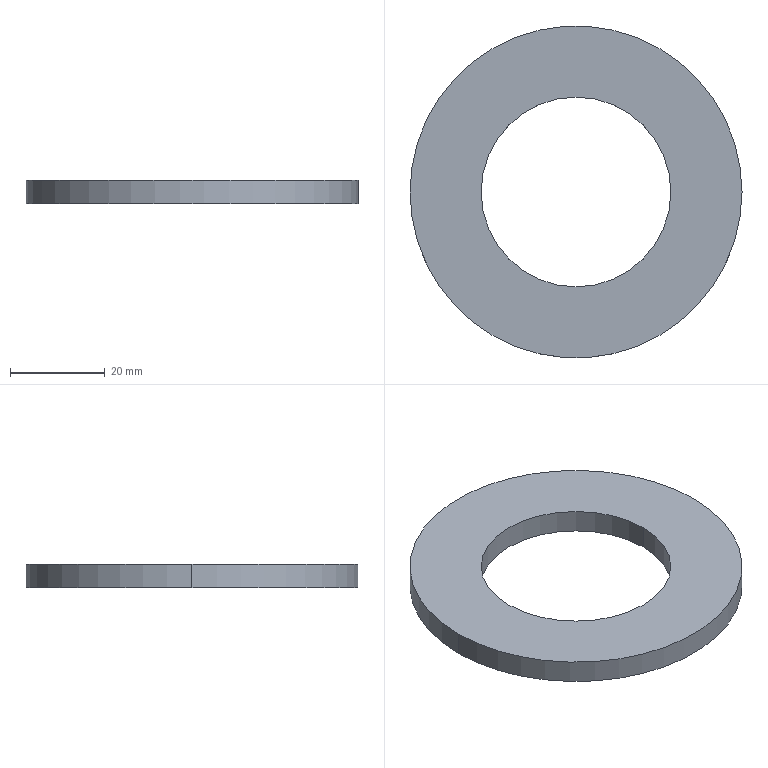Part | STEP file | 40 spacer XG | 1 solid | 6 faces | box 70 x 70 x 5 mm | volume 12959 mm3 | cylinder 4 | plane 2 | commonest cylinder face diameters 40 x2 70 x2
STEP:
#1=CARTESIAN_POINT('',(0.,0.,0.));
#2=DIRECTION('',(0.,0.,1.));
#3=DIRECTION('',(1.,0.,0.));
#4=AXIS2_PLACEMENT_3D('',#1,#2,#3);
#5=CARTESIAN_POINT('',(-20.,0.,5.));
#6=VERTEX_POINT('',#5);
#7=CARTESIAN_POINT('',(-20.,0.,0.));
#8=VERTEX_POINT('',#7);
#9=CARTESIAN_POINT('',(-20.,0.,5.));
#10=DIRECTION('',(0.,0.,-1.));
#11=VECTOR('',#10,1.);
#12=LINE('',#9,#11);
#13=CARTESIAN_POINT('',(0.,0.,5.));
#14=DIRECTION('',(0.,0.,-1.));
#15=DIRECTION('',(-1.,0.,0.));
#16=AXIS2_PLACEMENT_3D('',#13,#14,#15);
#17=CYLINDRICAL_SURFACE('',#16,20.);
#18=CARTESIAN_POINT('',(6.283,0.));
#19=DIRECTION('',(0.,1.));
#20=VECTOR('',#19,1.);
#21=LINE('',#18,#20);
#22=(GEOMETRIC_REPRESENTATION_CONTEXT(2)PARAMETRIC_REPRESENTATION_CONTEXT()REPRESENTATION_CONTEXT('',''));
#23=DEFINITIONAL_REPRESENTATION('',(#21),#22);
#24=PCURVE('',#17,#23);
#25=CARTESIAN_POINT('',(0.,0.,5.));
#26=DIRECTION('',(0.,0.,-1.));
#27=DIRECTION('',(-1.,0.,0.));
#28=AXIS2_PLACEMENT_3D('',#25,#26,#27);
#29=CYLINDRICAL_SURFACE('',#28,20.);
#30=CARTESIAN_POINT('',(0.,0.));
#31=DIRECTION('',(0.,1.));
#32=VECTOR('',#31,1.);
#33=LINE('',#30,#32);
#34=(GEOMETRIC_REPRESENTATION_CONTEXT(2)PARAMETRIC_REPRESENTATION_CONTEXT()REPRESENTATION_CONTEXT('',''));
#35=DEFINITIONAL_REPRESENTATION('',(#33),#34);
#36=PCURVE('',#29,#35);
#37=SURFACE_CURVE('',#12,(#24,#36),.PCURVE_S1.);
#38=EDGE_CURVE('',#6,#8,#37,.T.);
#39=ORIENTED_EDGE('',*,*,#38,.T.);
#40=CARTESIAN_POINT('',(20.,0.,0.));
#41=VERTEX_POINT('',#40);
#42=CARTESIAN_POINT('',(0.,0.,0.));
#43=DIRECTION('',(0.,0.,1.));
#44=DIRECTION('',(1.,0.,0.));
#45=AXIS2_PLACEMENT_3D('',#42,#43,#44);
#46=CIRCLE('',#45,20.);
#47=CARTESIAN_POINT('',(9.425,5.));
#48=DIRECTION('',(-1.,0.));
#49=VECTOR('',#48,1.);
#50=LINE('',#47,#49);
#51=(GEOMETRIC_REPRESENTATION_CONTEXT(2)PARAMETRIC_REPRESENTATION_CONTEXT()REPRESENTATION_CONTEXT('',''));
#52=DEFINITIONAL_REPRESENTATION('',(#50),#51);
#53=PCURVE('',#17,#52);
#54=CARTESIAN_POINT('',(0.,0.,0.));
#55=DIRECTION('',(0.,0.,1.));
#56=DIRECTION('',(1.,0.,0.));
#57=AXIS2_PLACEMENT_3D('',#54,#55,#56);
#58=PLANE('',#57);
#59=CARTESIAN_POINT('',(0.,0.));
#60=DIRECTION('',(1.,0.));
#61=AXIS2_PLACEMENT_2D('',#59,#60);
#62=CIRCLE('',#61,20.);
#63=(GEOMETRIC_REPRESENTATION_CONTEXT(2)PARAMETRIC_REPRESENTATION_CONTEXT()REPRESENTATION_CONTEXT('',''));
#64=DEFINITIONAL_REPRESENTATION('',(#62),#63);
#65=PCURVE('',#58,#64);
#66=SURFACE_CURVE('',#46,(#53,#65),.PCURVE_S1.);
#67=EDGE_CURVE('',#8,#41,#66,.T.);
#68=ORIENTED_EDGE('',*,*,#67,.T.);
#69=CARTESIAN_POINT('',(20.,0.,5.));
#70=VERTEX_POINT('',#69);
#71=CARTESIAN_POINT('',(20.,0.,5.));
#72=DIRECTION('',(0.,0.,-1.));
#73=VECTOR('',#72,1.);
#74=LINE('',#71,#73);
#75=CARTESIAN_POINT('',(3.142,0.));
#76=DIRECTION('',(0.,1.));
#77=VECTOR('',#76,1.);
#78=LINE('',#75,#77);
#79=(GEOMETRIC_REPRESENTATION_CONTEXT(2)PARAMETRIC_REPRESENTATION_CONTEXT()REPRESENTATION_CONTEXT('',''));
#80=DEFINITIONAL_REPRESENTATION('',(#78),#79);
#81=PCURVE('',#17,#80);
#82=CARTESIAN_POINT('',(3.142,0.));
#83=DIRECTION('',(0.,1.));
#84=VECTOR('',#83,1.);
#85=LINE('',#82,#84);
#86=(GEOMETRIC_REPRESENTATION_CONTEXT(2)PARAMETRIC_REPRESENTATION_CONTEXT()REPRESENTATION_CONTEXT('',''));
#87=DEFINITIONAL_REPRESENTATION('',(#85),#86);
#88=PCURVE('',#29,#87);
#89=SURFACE_CURVE('',#74,(#81,#88),.PCURVE_S1.);
#90=EDGE_CURVE('',#70,#41,#89,.T.);
#91=ORIENTED_EDGE('',*,*,#90,.F.);
#92=CARTESIAN_POINT('',(0.,0.,5.));
#93=DIRECTION('',(0.,0.,1.));
#94=DIRECTION('',(1.,0.,0.));
#95=AXIS2_PLACEMENT_3D('',#92,#93,#94);
#96=CIRCLE('',#95,20.);
#97=CARTESIAN_POINT('',(9.425,0.));
#98=DIRECTION('',(-1.,0.));
#99=VECTOR('',#98,1.);
#100=LINE('',#97,#99);
#101=(GEOMETRIC_REPRESENTATION_CONTEXT(2)PARAMETRIC_REPRESENTATION_CONTEXT()REPRESENTATION_CONTEXT('',''));
#102=DEFINITIONAL_REPRESENTATION('',(#100),#101);
#103=PCURVE('',#17,#102);
#104=CARTESIAN_POINT('',(0.,0.,5.));
#105=DIRECTION('',(0.,0.,1.));
#106=DIRECTION('',(1.,0.,0.));
#107=AXIS2_PLACEMENT_3D('',#104,#105,#106);
#108=PLANE('',#107);
#109=CARTESIAN_POINT('',(0.,0.));
#110=DIRECTION('',(1.,0.));
#111=AXIS2_PLACEMENT_2D('',#109,#110);
#112=CIRCLE('',#111,20.);
#113=(GEOMETRIC_REPRESENTATION_CONTEXT(2)PARAMETRIC_REPRESENTATION_CONTEXT()REPRESENTATION_CONTEXT('',''));
#114=DEFINITIONAL_REPRESENTATION('',(#112),#113);
#115=PCURVE('',#108,#114);
#116=SURFACE_CURVE('',#96,(#103,#115),.PCURVE_S1.);
#117=EDGE_CURVE('',#6,#70,#116,.T.);
#118=ORIENTED_EDGE('',*,*,#117,.F.);
#119=EDGE_LOOP('',(#39,#68,#91,#118));
#120=FACE_BOUND('',#119,.F.);
#121=ADVANCED_FACE('',(#120),#17,.F.);
#122=CARTESIAN_POINT('',(35.,0.,5.));
#123=VERTEX_POINT('',#122);
#124=CARTESIAN_POINT('',(-35.,0.,5.));
#125=VERTEX_POINT('',#124);
#126=CARTESIAN_POINT('',(0.,0.,5.));
#127=DIRECTION('',(0.,0.,1.));
#128=DIRECTION('',(1.,0.,0.));
#129=AXIS2_PLACEMENT_3D('',#126,#127,#128);
#130=CIRCLE('',#129,35.);
#131=CARTESIAN_POINT('',(0.,0.,5.));
#132=DIRECTION('',(0.,0.,-1.));
#133=DIRECTION('',(-1.,0.,0.));
#134=AXIS2_PLACEMENT_3D('',#131,#132,#133);
#135=CYLINDRICAL_SURFACE('',#134,35.);
#136=CARTESIAN_POINT('',(3.142,0.));
#137=DIRECTION('',(-1.,0.));
#138=VECTOR('',#137,1.);
#139=LINE('',#136,#138);
#140=(GEOMETRIC_REPRESENTATION_CONTEXT(2)PARAMETRIC_REPRESENTATION_CONTEXT()REPRESENTATION_CONTEXT('',''));
#141=DEFINITIONAL_REPRESENTATION('',(#139),#140);
#142=PCURVE('',#135,#141);
#143=CARTESIAN_POINT('',(0.,0.));
#144=DIRECTION('',(1.,0.));
#145=AXIS2_PLACEMENT_2D('',#143,#144);
#146=CIRCLE('',#145,35.);
#147=(GEOMETRIC_REPRESENTATION_CONTEXT(2)PARAMETRIC_REPRESENTATION_CONTEXT()REPRESENTATION_CONTEXT('',''));
#148=DEFINITIONAL_REPRESENTATION('',(#146),#147);
#149=PCURVE('',#108,#148);
#150=SURFACE_CURVE('',#130,(#142,#149),.PCURVE_S1.);
#151=EDGE_CURVE('',#123,#125,#150,.T.);
#152=ORIENTED_EDGE('',*,*,#151,.F.);
#153=CARTESIAN_POINT('',(35.,0.,0.));
#154=VERTEX_POINT('',#153);
#155=CARTESIAN_POINT('',(35.,0.,5.));
#156=DIRECTION('',(0.,0.,-1.));
#157=VECTOR('',#156,1.);
#158=LINE('',#155,#157);
#159=CARTESIAN_POINT('',(3.142,0.));
#160=DIRECTION('',(0.,1.));
#161=VECTOR('',#160,1.);
#162=LINE('',#159,#161);
#163=(GEOMETRIC_REPRESENTATION_CONTEXT(2)PARAMETRIC_REPRESENTATION_CONTEXT()REPRESENTATION_CONTEXT('',''));
#164=DEFINITIONAL_REPRESENTATION('',(#162),#163);
#165=PCURVE('',#135,#164);
#166=CARTESIAN_POINT('',(0.,0.,5.));
#167=DIRECTION('',(0.,0.,-1.));
#168=DIRECTION('',(-1.,0.,0.));
#169=AXIS2_PLACEMENT_3D('',#166,#167,#168);
#170=CYLINDRICAL_SURFACE('',#169,35.);
#171=CARTESIAN_POINT('',(3.142,0.));
#172=DIRECTION('',(0.,1.));
#173=VECTOR('',#172,1.);
#174=LINE('',#171,#173);
#175=(GEOMETRIC_REPRESENTATION_CONTEXT(2)PARAMETRIC_REPRESENTATION_CONTEXT()REPRESENTATION_CONTEXT('',''));
#176=DEFINITIONAL_REPRESENTATION('',(#174),#175);
#177=PCURVE('',#170,#176);
#178=SURFACE_CURVE('',#158,(#165,#177),.PCURVE_S1.);
#179=EDGE_CURVE('',#123,#154,#178,.T.);
#180=ORIENTED_EDGE('',*,*,#179,.T.);
#181=CARTESIAN_POINT('',(-35.,0.,0.));
#182=VERTEX_POINT('',#181);
#183=CARTESIAN_POINT('',(0.,0.,0.));
#184=DIRECTION('',(0.,0.,1.));
#185=DIRECTION('',(1.,0.,0.));
#186=AXIS2_PLACEMENT_3D('',#183,#184,#185);
#187=CIRCLE('',#186,35.);
#188=CARTESIAN_POINT('',(3.142,5.));
#189=DIRECTION('',(-1.,0.));
#190=VECTOR('',#189,1.);
#191=LINE('',#188,#190);
#192=(GEOMETRIC_REPRESENTATION_CONTEXT(2)PARAMETRIC_REPRESENTATION_CONTEXT()REPRESENTATION_CONTEXT('',''));
#193=DEFINITIONAL_REPRESENTATION('',(#191),#192);
#194=PCURVE('',#135,#193);
#195=CARTESIAN_POINT('',(0.,0.));
#196=DIRECTION('',(1.,0.));
#197=AXIS2_PLACEMENT_2D('',#195,#196);
#198=CIRCLE('',#197,35.);
#199=(GEOMETRIC_REPRESENTATION_CONTEXT(2)PARAMETRIC_REPRESENTATION_CONTEXT()REPRESENTATION_CONTEXT('',''));
#200=DEFINITIONAL_REPRESENTATION('',(#198),#199);
#201=PCURVE('',#58,#200);
#202=SURFACE_CURVE('',#187,(#194,#201),.PCURVE_S1.);
#203=EDGE_CURVE('',#154,#182,#202,.T.);
#204=ORIENTED_EDGE('',*,*,#203,.T.);
#205=CARTESIAN_POINT('',(-35.,0.,5.));
#206=DIRECTION('',(0.,0.,-1.));
#207=VECTOR('',#206,1.);
#208=LINE('',#205,#207);
#209=CARTESIAN_POINT('',(0.,0.));
#210=DIRECTION('',(0.,1.));
#211=VECTOR('',#210,1.);
#212=LINE('',#209,#211);
#213=(GEOMETRIC_REPRESENTATION_CONTEXT(2)PARAMETRIC_REPRESENTATION_CONTEXT()REPRESENTATION_CONTEXT('',''));
#214=DEFINITIONAL_REPRESENTATION('',(#212),#213);
#215=PCURVE('',#135,#214);
#216=CARTESIAN_POINT('',(6.283,0.));
#217=DIRECTION('',(0.,1.));
#218=VECTOR('',#217,1.);
#219=LINE('',#216,#218);
#220=(GEOMETRIC_REPRESENTATION_CONTEXT(2)PARAMETRIC_REPRESENTATION_CONTEXT()REPRESENTATION_CONTEXT('',''));
#221=DEFINITIONAL_REPRESENTATION('',(#219),#220);
#222=PCURVE('',#170,#221);
#223=SURFACE_CURVE('',#208,(#215,#222),.PCURVE_S1.);
#224=EDGE_CURVE('',#125,#182,#223,.T.);
#225=ORIENTED_EDGE('',*,*,#224,.F.);
#226=EDGE_LOOP('',(#152,#180,#204,#225));
#227=FACE_BOUND('',#226,.T.);
#228=ADVANCED_FACE('',(#227),#135,.T.);
#229=CARTESIAN_POINT('',(0.,0.,5.));
#230=DIRECTION('',(0.,0.,1.));
#231=DIRECTION('',(1.,0.,0.));
#232=AXIS2_PLACEMENT_3D('',#229,#230,#231);
#233=CIRCLE('',#232,35.);
#234=CARTESIAN_POINT('',(0.,0.));
#235=DIRECTION('',(1.,0.));
#236=AXIS2_PLACEMENT_2D('',#234,#235);
#237=CIRCLE('',#236,35.);
#238=(GEOMETRIC_REPRESENTATION_CONTEXT(2)PARAMETRIC_REPRESENTATION_CONTEXT()REPRESENTATION_CONTEXT('',''));
#239=DEFINITIONAL_REPRESENTATION('',(#237),#238);
#240=PCURVE('',#108,#239);
#241=CARTESIAN_POINT('',(9.425,0.));
#242=DIRECTION('',(-1.,0.));
#243=VECTOR('',#242,1.);
#244=LINE('',#241,#243);
#245=(GEOMETRIC_REPRESENTATION_CONTEXT(2)PARAMETRIC_REPRESENTATION_CONTEXT()REPRESENTATION_CONTEXT('',''));
#246=DEFINITIONAL_REPRESENTATION('',(#244),#245);
#247=PCURVE('',#170,#246);
#248=SURFACE_CURVE('',#233,(#240,#247),.PCURVE_S1.);
#249=EDGE_CURVE('',#125,#123,#248,.T.);
#250=ORIENTED_EDGE('',*,*,#249,.T.);
#251=ORIENTED_EDGE('',*,*,#151,.T.);
#252=EDGE_LOOP('',(#250,#251));
#253=FACE_BOUND('',#252,.T.);
#254=ORIENTED_EDGE('',*,*,#117,.F.);
#255=CARTESIAN_POINT('',(0.,0.,5.));
#256=DIRECTION('',(0.,0.,1.));
#257=DIRECTION('',(1.,0.,0.));
#258=AXIS2_PLACEMENT_3D('',#255,#256,#257);
#259=CIRCLE('',#258,20.);
#260=CARTESIAN_POINT('',(0.,0.));
#261=DIRECTION('',(1.,0.));
#262=AXIS2_PLACEMENT_2D('',#260,#261);
#263=CIRCLE('',#262,20.);
#264=(GEOMETRIC_REPRESENTATION_CONTEXT(2)PARAMETRIC_REPRESENTATION_CONTEXT()REPRESENTATION_CONTEXT('',''));
#265=DEFINITIONAL_REPRESENTATION('',(#263),#264);
#266=PCURVE('',#108,#265);
#267=CARTESIAN_POINT('',(3.142,0.));
#268=DIRECTION('',(-1.,0.));
#269=VECTOR('',#268,1.);
#270=LINE('',#267,#269);
#271=(GEOMETRIC_REPRESENTATION_CONTEXT(2)PARAMETRIC_REPRESENTATION_CONTEXT()REPRESENTATION_CONTEXT('',''));
#272=DEFINITIONAL_REPRESENTATION('',(#270),#271);
#273=PCURVE('',#29,#272);
#274=SURFACE_CURVE('',#259,(#266,#273),.PCURVE_S1.);
#275=EDGE_CURVE('',#70,#6,#274,.T.);
#276=ORIENTED_EDGE('',*,*,#275,.F.);
#277=EDGE_LOOP('',(#254,#276));
#278=FACE_BOUND('',#277,.T.);
#279=ADVANCED_FACE('',(#253,#278),#108,.T.);
#280=CARTESIAN_POINT('',(0.,0.,0.));
#281=DIRECTION('',(0.,0.,1.));
#282=DIRECTION('',(1.,0.,0.));
#283=AXIS2_PLACEMENT_3D('',#280,#281,#282);
#284=CIRCLE('',#283,35.);
#285=CARTESIAN_POINT('',(0.,0.));
#286=DIRECTION('',(1.,0.));
#287=AXIS2_PLACEMENT_2D('',#285,#286);
#288=CIRCLE('',#287,35.);
#289=(GEOMETRIC_REPRESENTATION_CONTEXT(2)PARAMETRIC_REPRESENTATION_CONTEXT()REPRESENTATION_CONTEXT('',''));
#290=DEFINITIONAL_REPRESENTATION('',(#288),#289);
#291=PCURVE('',#58,#290);
#292=CARTESIAN_POINT('',(9.425,5.));
#293=DIRECTION('',(-1.,0.));
#294=VECTOR('',#293,1.);
#295=LINE('',#292,#294);
#296=(GEOMETRIC_REPRESENTATION_CONTEXT(2)PARAMETRIC_REPRESENTATION_CONTEXT()REPRESENTATION_CONTEXT('',''));
#297=DEFINITIONAL_REPRESENTATION('',(#295),#296);
#298=PCURVE('',#170,#297);
#299=SURFACE_CURVE('',#284,(#291,#298),.PCURVE_S1.);
#300=EDGE_CURVE('',#182,#154,#299,.T.);
#301=ORIENTED_EDGE('',*,*,#300,.F.);
#302=ORIENTED_EDGE('',*,*,#203,.F.);
#303=EDGE_LOOP('',(#301,#302));
#304=FACE_BOUND('',#303,.T.);
#305=ORIENTED_EDGE('',*,*,#67,.T.);
#306=CARTESIAN_POINT('',(0.,0.,0.));
#307=DIRECTION('',(0.,0.,1.));
#308=DIRECTION('',(1.,0.,0.));
#309=AXIS2_PLACEMENT_3D('',#306,#307,#308);
#310=CIRCLE('',#309,20.);
#311=CARTESIAN_POINT('',(0.,0.));
#312=DIRECTION('',(1.,0.));
#313=AXIS2_PLACEMENT_2D('',#311,#312);
#314=CIRCLE('',#313,20.);
#315=(GEOMETRIC_REPRESENTATION_CONTEXT(2)PARAMETRIC_REPRESENTATION_CONTEXT()REPRESENTATION_CONTEXT('',''));
#316=DEFINITIONAL_REPRESENTATION('',(#314),#315);
#317=PCURVE('',#58,#316);
#318=CARTESIAN_POINT('',(3.142,5.));
#319=DIRECTION('',(-1.,0.));
#320=VECTOR('',#319,1.);
#321=LINE('',#318,#320);
#322=(GEOMETRIC_REPRESENTATION_CONTEXT(2)PARAMETRIC_REPRESENTATION_CONTEXT()REPRESENTATION_CONTEXT('',''));
#323=DEFINITIONAL_REPRESENTATION('',(#321),#322);
#324=PCURVE('',#29,#323);
#325=SURFACE_CURVE('',#310,(#317,#324),.PCURVE_S1.);
#326=EDGE_CURVE('',#41,#8,#325,.T.);
#327=ORIENTED_EDGE('',*,*,#326,.T.);
#328=EDGE_LOOP('',(#305,#327));
#329=FACE_BOUND('',#328,.T.);
#330=ADVANCED_FACE('',(#304,#329),#58,.F.);
#331=ORIENTED_EDGE('',*,*,#179,.F.);
#332=ORIENTED_EDGE('',*,*,#249,.F.);
#333=ORIENTED_EDGE('',*,*,#224,.T.);
#334=ORIENTED_EDGE('',*,*,#300,.T.);
#335=EDGE_LOOP('',(#331,#332,#333,#334));
#336=FACE_BOUND('',#335,.T.);
#337=ADVANCED_FACE('',(#336),#170,.T.);
#338=ORIENTED_EDGE('',*,*,#326,.T.);
#339=ORIENTED_EDGE('',*,*,#38,.F.);
#340=ORIENTED_EDGE('',*,*,#275,.F.);
#341=ORIENTED_EDGE('',*,*,#90,.T.);
#342=EDGE_LOOP('',(#338,#339,#340,#341));
#343=FACE_BOUND('',#342,.F.);
#344=ADVANCED_FACE('',(#343),#29,.F.);
#345=CLOSED_SHELL('',(#121,#228,#279,#330,#337,#344));
#346=MANIFOLD_SOLID_BREP('',#345);
#347=(LENGTH_UNIT()NAMED_UNIT(*)SI_UNIT(.MILLI.,.METRE.));
#348=UNCERTAINTY_MEASURE_WITH_UNIT(LENGTH_MEASURE(0.0000001),#347,'','');
#349=(NAMED_UNIT(*)PLANE_ANGLE_UNIT()SI_UNIT($,.RADIAN.));
#350=(NAMED_UNIT(*)SI_UNIT($,.STERADIAN.)SOLID_ANGLE_UNIT());
#351=(GEOMETRIC_REPRESENTATION_CONTEXT(3)GLOBAL_UNCERTAINTY_ASSIGNED_CONTEXT((#348))GLOBAL_UNIT_ASSIGNED_CONTEXT((#347,#349,#350))REPRESENTATION_CONTEXT('',''));
#352=ADVANCED_BREP_SHAPE_REPRESENTATION('',(#4,#346),#351);